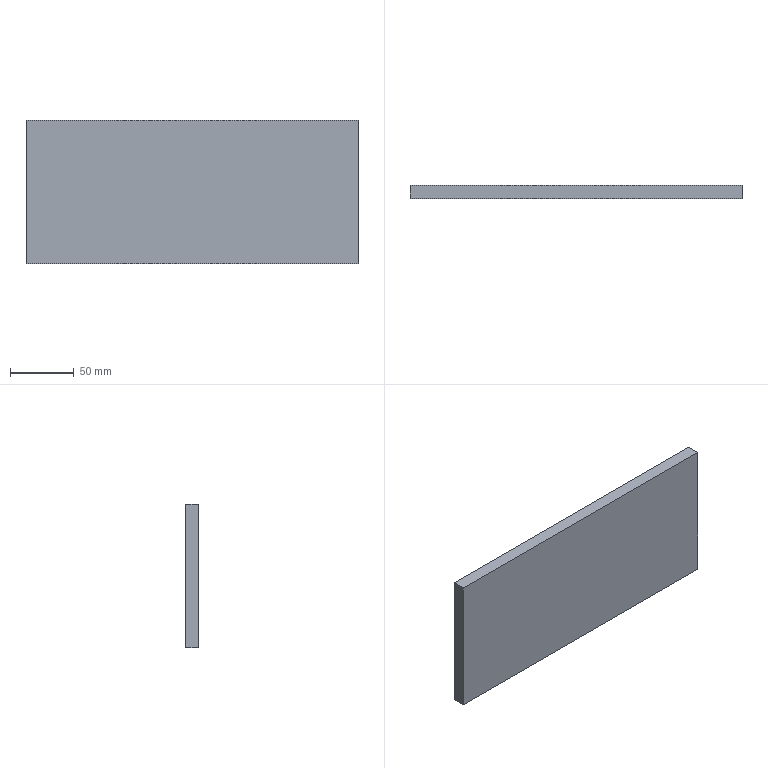Part | STEP file | Drawer | 1 solid | 6 faces | box 260 x 10 x 112 mm | volume 291200 mm3 | plane 6
STEP:
#1=CARTESIAN_POINT('',(0.,0.,0.));
#2=DIRECTION('',(0.,0.,1.));
#3=DIRECTION('',(1.,0.,0.));
#4=AXIS2_PLACEMENT_3D('',#1,#2,#3);
#5=CARTESIAN_POINT('',(-130.,0.,112.));
#6=VERTEX_POINT('',#5);
#7=CARTESIAN_POINT('',(-130.,-10.,112.));
#8=VERTEX_POINT('',#7);
#9=CARTESIAN_POINT('',(-130.,0.,112.));
#10=DIRECTION('',(0.,-1.,0.));
#11=VECTOR('',#10,1.);
#12=LINE('',#9,#11);
#13=CARTESIAN_POINT('',(-130.,0.,112.));
#14=DIRECTION('',(1.,0.,0.));
#15=DIRECTION('',(0.,0.,-1.));
#16=AXIS2_PLACEMENT_3D('',#13,#14,#15);
#17=PLANE('',#16);
#18=CARTESIAN_POINT('',(0.,0.));
#19=DIRECTION('',(0.,-1.));
#20=VECTOR('',#19,1.);
#21=LINE('',#18,#20);
#22=(GEOMETRIC_REPRESENTATION_CONTEXT(2)PARAMETRIC_REPRESENTATION_CONTEXT()REPRESENTATION_CONTEXT('',''));
#23=DEFINITIONAL_REPRESENTATION('',(#21),#22);
#24=PCURVE('',#17,#23);
#25=CARTESIAN_POINT('',(130.,0.,112.));
#26=DIRECTION('',(0.,0.,-1.));
#27=DIRECTION('',(-1.,0.,0.));
#28=AXIS2_PLACEMENT_3D('',#25,#26,#27);
#29=PLANE('',#28);
#30=CARTESIAN_POINT('',(260.,0.));
#31=DIRECTION('',(0.,-1.));
#32=VECTOR('',#31,1.);
#33=LINE('',#30,#32);
#34=(GEOMETRIC_REPRESENTATION_CONTEXT(2)PARAMETRIC_REPRESENTATION_CONTEXT()REPRESENTATION_CONTEXT('',''));
#35=DEFINITIONAL_REPRESENTATION('',(#33),#34);
#36=PCURVE('',#29,#35);
#37=SURFACE_CURVE('',#12,(#24,#36),.PCURVE_S1.);
#38=EDGE_CURVE('',#6,#8,#37,.T.);
#39=ORIENTED_EDGE('',*,*,#38,.T.);
#40=CARTESIAN_POINT('',(-130.,-10.,0.));
#41=VERTEX_POINT('',#40);
#42=CARTESIAN_POINT('',(-130.,-10.,112.));
#43=DIRECTION('',(0.,0.,-1.));
#44=VECTOR('',#43,1.);
#45=LINE('',#42,#44);
#46=CARTESIAN_POINT('',(0.,-10.));
#47=DIRECTION('',(1.,0.));
#48=VECTOR('',#47,1.);
#49=LINE('',#46,#48);
#50=(GEOMETRIC_REPRESENTATION_CONTEXT(2)PARAMETRIC_REPRESENTATION_CONTEXT()REPRESENTATION_CONTEXT('',''));
#51=DEFINITIONAL_REPRESENTATION('',(#49),#50);
#52=PCURVE('',#17,#51);
#53=CARTESIAN_POINT('',(0.,-10.,56.));
#54=DIRECTION('',(0.,1.,0.));
#55=DIRECTION('',(0.,0.,1.));
#56=AXIS2_PLACEMENT_3D('',#53,#54,#55);
#57=PLANE('',#56);
#58=CARTESIAN_POINT('',(56.,-130.));
#59=DIRECTION('',(-1.,0.));
#60=VECTOR('',#59,1.);
#61=LINE('',#58,#60);
#62=(GEOMETRIC_REPRESENTATION_CONTEXT(2)PARAMETRIC_REPRESENTATION_CONTEXT()REPRESENTATION_CONTEXT('',''));
#63=DEFINITIONAL_REPRESENTATION('',(#61),#62);
#64=PCURVE('',#57,#63);
#65=SURFACE_CURVE('',#45,(#52,#64),.PCURVE_S1.);
#66=EDGE_CURVE('',#8,#41,#65,.T.);
#67=ORIENTED_EDGE('',*,*,#66,.T.);
#68=CARTESIAN_POINT('',(-130.,0.,0.));
#69=VERTEX_POINT('',#68);
#70=CARTESIAN_POINT('',(-130.,0.,0.));
#71=DIRECTION('',(0.,-1.,0.));
#72=VECTOR('',#71,1.);
#73=LINE('',#70,#72);
#74=CARTESIAN_POINT('',(112.,0.));
#75=DIRECTION('',(0.,-1.));
#76=VECTOR('',#75,1.);
#77=LINE('',#74,#76);
#78=(GEOMETRIC_REPRESENTATION_CONTEXT(2)PARAMETRIC_REPRESENTATION_CONTEXT()REPRESENTATION_CONTEXT('',''));
#79=DEFINITIONAL_REPRESENTATION('',(#77),#78);
#80=PCURVE('',#17,#79);
#81=CARTESIAN_POINT('',(-130.,0.,0.));
#82=DIRECTION('',(0.,0.,1.));
#83=DIRECTION('',(1.,0.,0.));
#84=AXIS2_PLACEMENT_3D('',#81,#82,#83);
#85=PLANE('',#84);
#86=CARTESIAN_POINT('',(0.,0.));
#87=DIRECTION('',(0.,-1.));
#88=VECTOR('',#87,1.);
#89=LINE('',#86,#88);
#90=(GEOMETRIC_REPRESENTATION_CONTEXT(2)PARAMETRIC_REPRESENTATION_CONTEXT()REPRESENTATION_CONTEXT('',''));
#91=DEFINITIONAL_REPRESENTATION('',(#89),#90);
#92=PCURVE('',#85,#91);
#93=SURFACE_CURVE('',#73,(#80,#92),.PCURVE_S1.);
#94=EDGE_CURVE('',#69,#41,#93,.T.);
#95=ORIENTED_EDGE('',*,*,#94,.F.);
#96=CARTESIAN_POINT('',(-130.,0.,112.));
#97=DIRECTION('',(0.,0.,-1.));
#98=VECTOR('',#97,1.);
#99=LINE('',#96,#98);
#100=CARTESIAN_POINT('',(0.,0.));
#101=DIRECTION('',(1.,0.));
#102=VECTOR('',#101,1.);
#103=LINE('',#100,#102);
#104=(GEOMETRIC_REPRESENTATION_CONTEXT(2)PARAMETRIC_REPRESENTATION_CONTEXT()REPRESENTATION_CONTEXT('',''));
#105=DEFINITIONAL_REPRESENTATION('',(#103),#104);
#106=PCURVE('',#17,#105);
#107=CARTESIAN_POINT('',(0.,0.,56.));
#108=DIRECTION('',(0.,1.,0.));
#109=DIRECTION('',(0.,0.,1.));
#110=AXIS2_PLACEMENT_3D('',#107,#108,#109);
#111=PLANE('',#110);
#112=CARTESIAN_POINT('',(56.,-130.));
#113=DIRECTION('',(-1.,0.));
#114=VECTOR('',#113,1.);
#115=LINE('',#112,#114);
#116=(GEOMETRIC_REPRESENTATION_CONTEXT(2)PARAMETRIC_REPRESENTATION_CONTEXT()REPRESENTATION_CONTEXT('',''));
#117=DEFINITIONAL_REPRESENTATION('',(#115),#116);
#118=PCURVE('',#111,#117);
#119=SURFACE_CURVE('',#99,(#106,#118),.PCURVE_S1.);
#120=EDGE_CURVE('',#6,#69,#119,.T.);
#121=ORIENTED_EDGE('',*,*,#120,.F.);
#122=EDGE_LOOP('',(#39,#67,#95,#121));
#123=FACE_BOUND('',#122,.F.);
#124=ADVANCED_FACE('',(#123),#17,.F.);
#125=ORIENTED_EDGE('',*,*,#94,.T.);
#126=CARTESIAN_POINT('',(130.,-10.,0.));
#127=VERTEX_POINT('',#126);
#128=CARTESIAN_POINT('',(-130.,-10.,0.));
#129=DIRECTION('',(1.,0.,0.));
#130=VECTOR('',#129,1.);
#131=LINE('',#128,#130);
#132=CARTESIAN_POINT('',(0.,-10.));
#133=DIRECTION('',(1.,0.));
#134=VECTOR('',#133,1.);
#135=LINE('',#132,#134);
#136=(GEOMETRIC_REPRESENTATION_CONTEXT(2)PARAMETRIC_REPRESENTATION_CONTEXT()REPRESENTATION_CONTEXT('',''));
#137=DEFINITIONAL_REPRESENTATION('',(#135),#136);
#138=PCURVE('',#85,#137);
#139=CARTESIAN_POINT('',(-56.,-130.));
#140=DIRECTION('',(0.,1.));
#141=VECTOR('',#140,1.);
#142=LINE('',#139,#141);
#143=(GEOMETRIC_REPRESENTATION_CONTEXT(2)PARAMETRIC_REPRESENTATION_CONTEXT()REPRESENTATION_CONTEXT('',''));
#144=DEFINITIONAL_REPRESENTATION('',(#142),#143);
#145=PCURVE('',#57,#144);
#146=SURFACE_CURVE('',#131,(#138,#145),.PCURVE_S1.);
#147=EDGE_CURVE('',#41,#127,#146,.T.);
#148=ORIENTED_EDGE('',*,*,#147,.T.);
#149=CARTESIAN_POINT('',(130.,0.,0.));
#150=VERTEX_POINT('',#149);
#151=CARTESIAN_POINT('',(130.,0.,0.));
#152=DIRECTION('',(0.,-1.,0.));
#153=VECTOR('',#152,1.);
#154=LINE('',#151,#153);
#155=CARTESIAN_POINT('',(260.,0.));
#156=DIRECTION('',(0.,-1.));
#157=VECTOR('',#156,1.);
#158=LINE('',#155,#157);
#159=(GEOMETRIC_REPRESENTATION_CONTEXT(2)PARAMETRIC_REPRESENTATION_CONTEXT()REPRESENTATION_CONTEXT('',''));
#160=DEFINITIONAL_REPRESENTATION('',(#158),#159);
#161=PCURVE('',#85,#160);
#162=CARTESIAN_POINT('',(130.,0.,0.));
#163=DIRECTION('',(-1.,0.,0.));
#164=DIRECTION('',(0.,0.,1.));
#165=AXIS2_PLACEMENT_3D('',#162,#163,#164);
#166=PLANE('',#165);
#167=CARTESIAN_POINT('',(0.,0.));
#168=DIRECTION('',(0.,-1.));
#169=VECTOR('',#168,1.);
#170=LINE('',#167,#169);
#171=(GEOMETRIC_REPRESENTATION_CONTEXT(2)PARAMETRIC_REPRESENTATION_CONTEXT()REPRESENTATION_CONTEXT('',''));
#172=DEFINITIONAL_REPRESENTATION('',(#170),#171);
#173=PCURVE('',#166,#172);
#174=SURFACE_CURVE('',#154,(#161,#173),.PCURVE_S1.);
#175=EDGE_CURVE('',#150,#127,#174,.T.);
#176=ORIENTED_EDGE('',*,*,#175,.F.);
#177=CARTESIAN_POINT('',(-130.,0.,0.));
#178=DIRECTION('',(1.,0.,0.));
#179=VECTOR('',#178,1.);
#180=LINE('',#177,#179);
#181=CARTESIAN_POINT('',(0.,0.));
#182=DIRECTION('',(1.,0.));
#183=VECTOR('',#182,1.);
#184=LINE('',#181,#183);
#185=(GEOMETRIC_REPRESENTATION_CONTEXT(2)PARAMETRIC_REPRESENTATION_CONTEXT()REPRESENTATION_CONTEXT('',''));
#186=DEFINITIONAL_REPRESENTATION('',(#184),#185);
#187=PCURVE('',#85,#186);
#188=CARTESIAN_POINT('',(-56.,-130.));
#189=DIRECTION('',(0.,1.));
#190=VECTOR('',#189,1.);
#191=LINE('',#188,#190);
#192=(GEOMETRIC_REPRESENTATION_CONTEXT(2)PARAMETRIC_REPRESENTATION_CONTEXT()REPRESENTATION_CONTEXT('',''));
#193=DEFINITIONAL_REPRESENTATION('',(#191),#192);
#194=PCURVE('',#111,#193);
#195=SURFACE_CURVE('',#180,(#187,#194),.PCURVE_S1.);
#196=EDGE_CURVE('',#69,#150,#195,.T.);
#197=ORIENTED_EDGE('',*,*,#196,.F.);
#198=EDGE_LOOP('',(#125,#148,#176,#197));
#199=FACE_BOUND('',#198,.F.);
#200=ADVANCED_FACE('',(#199),#85,.F.);
#201=ORIENTED_EDGE('',*,*,#175,.T.);
#202=CARTESIAN_POINT('',(130.,-10.,112.));
#203=VERTEX_POINT('',#202);
#204=CARTESIAN_POINT('',(130.,-10.,0.));
#205=DIRECTION('',(0.,0.,1.));
#206=VECTOR('',#205,1.);
#207=LINE('',#204,#206);
#208=CARTESIAN_POINT('',(0.,-10.));
#209=DIRECTION('',(1.,0.));
#210=VECTOR('',#209,1.);
#211=LINE('',#208,#210);
#212=(GEOMETRIC_REPRESENTATION_CONTEXT(2)PARAMETRIC_REPRESENTATION_CONTEXT()REPRESENTATION_CONTEXT('',''));
#213=DEFINITIONAL_REPRESENTATION('',(#211),#212);
#214=PCURVE('',#166,#213);
#215=CARTESIAN_POINT('',(-56.,130.));
#216=DIRECTION('',(1.,0.));
#217=VECTOR('',#216,1.);
#218=LINE('',#215,#217);
#219=(GEOMETRIC_REPRESENTATION_CONTEXT(2)PARAMETRIC_REPRESENTATION_CONTEXT()REPRESENTATION_CONTEXT('',''));
#220=DEFINITIONAL_REPRESENTATION('',(#218),#219);
#221=PCURVE('',#57,#220);
#222=SURFACE_CURVE('',#207,(#214,#221),.PCURVE_S1.);
#223=EDGE_CURVE('',#127,#203,#222,.T.);
#224=ORIENTED_EDGE('',*,*,#223,.T.);
#225=CARTESIAN_POINT('',(130.,0.,112.));
#226=VERTEX_POINT('',#225);
#227=CARTESIAN_POINT('',(130.,0.,112.));
#228=DIRECTION('',(0.,-1.,0.));
#229=VECTOR('',#228,1.);
#230=LINE('',#227,#229);
#231=CARTESIAN_POINT('',(112.,0.));
#232=DIRECTION('',(0.,-1.));
#233=VECTOR('',#232,1.);
#234=LINE('',#231,#233);
#235=(GEOMETRIC_REPRESENTATION_CONTEXT(2)PARAMETRIC_REPRESENTATION_CONTEXT()REPRESENTATION_CONTEXT('',''));
#236=DEFINITIONAL_REPRESENTATION('',(#234),#235);
#237=PCURVE('',#166,#236);
#238=CARTESIAN_POINT('',(0.,0.));
#239=DIRECTION('',(0.,-1.));
#240=VECTOR('',#239,1.);
#241=LINE('',#238,#240);
#242=(GEOMETRIC_REPRESENTATION_CONTEXT(2)PARAMETRIC_REPRESENTATION_CONTEXT()REPRESENTATION_CONTEXT('',''));
#243=DEFINITIONAL_REPRESENTATION('',(#241),#242);
#244=PCURVE('',#29,#243);
#245=SURFACE_CURVE('',#230,(#237,#244),.PCURVE_S1.);
#246=EDGE_CURVE('',#226,#203,#245,.T.);
#247=ORIENTED_EDGE('',*,*,#246,.F.);
#248=CARTESIAN_POINT('',(130.,0.,0.));
#249=DIRECTION('',(0.,0.,1.));
#250=VECTOR('',#249,1.);
#251=LINE('',#248,#250);
#252=CARTESIAN_POINT('',(0.,0.));
#253=DIRECTION('',(1.,0.));
#254=VECTOR('',#253,1.);
#255=LINE('',#252,#254);
#256=(GEOMETRIC_REPRESENTATION_CONTEXT(2)PARAMETRIC_REPRESENTATION_CONTEXT()REPRESENTATION_CONTEXT('',''));
#257=DEFINITIONAL_REPRESENTATION('',(#255),#256);
#258=PCURVE('',#166,#257);
#259=CARTESIAN_POINT('',(-56.,130.));
#260=DIRECTION('',(1.,0.));
#261=VECTOR('',#260,1.);
#262=LINE('',#259,#261);
#263=(GEOMETRIC_REPRESENTATION_CONTEXT(2)PARAMETRIC_REPRESENTATION_CONTEXT()REPRESENTATION_CONTEXT('',''));
#264=DEFINITIONAL_REPRESENTATION('',(#262),#263);
#265=PCURVE('',#111,#264);
#266=SURFACE_CURVE('',#251,(#258,#265),.PCURVE_S1.);
#267=EDGE_CURVE('',#150,#226,#266,.T.);
#268=ORIENTED_EDGE('',*,*,#267,.F.);
#269=EDGE_LOOP('',(#201,#224,#247,#268));
#270=FACE_BOUND('',#269,.F.);
#271=ADVANCED_FACE('',(#270),#166,.F.);
#272=ORIENTED_EDGE('',*,*,#246,.T.);
#273=CARTESIAN_POINT('',(130.,-10.,112.));
#274=DIRECTION('',(-1.,0.,0.));
#275=VECTOR('',#274,1.);
#276=LINE('',#273,#275);
#277=CARTESIAN_POINT('',(0.,-10.));
#278=DIRECTION('',(1.,0.));
#279=VECTOR('',#278,1.);
#280=LINE('',#277,#279);
#281=(GEOMETRIC_REPRESENTATION_CONTEXT(2)PARAMETRIC_REPRESENTATION_CONTEXT()REPRESENTATION_CONTEXT('',''));
#282=DEFINITIONAL_REPRESENTATION('',(#280),#281);
#283=PCURVE('',#29,#282);
#284=CARTESIAN_POINT('',(56.,130.));
#285=DIRECTION('',(0.,-1.));
#286=VECTOR('',#285,1.);
#287=LINE('',#284,#286);
#288=(GEOMETRIC_REPRESENTATION_CONTEXT(2)PARAMETRIC_REPRESENTATION_CONTEXT()REPRESENTATION_CONTEXT('',''));
#289=DEFINITIONAL_REPRESENTATION('',(#287),#288);
#290=PCURVE('',#57,#289);
#291=SURFACE_CURVE('',#276,(#283,#290),.PCURVE_S1.);
#292=EDGE_CURVE('',#203,#8,#291,.T.);
#293=ORIENTED_EDGE('',*,*,#292,.T.);
#294=ORIENTED_EDGE('',*,*,#38,.F.);
#295=CARTESIAN_POINT('',(130.,0.,112.));
#296=DIRECTION('',(-1.,0.,0.));
#297=VECTOR('',#296,1.);
#298=LINE('',#295,#297);
#299=CARTESIAN_POINT('',(0.,0.));
#300=DIRECTION('',(1.,0.));
#301=VECTOR('',#300,1.);
#302=LINE('',#299,#301);
#303=(GEOMETRIC_REPRESENTATION_CONTEXT(2)PARAMETRIC_REPRESENTATION_CONTEXT()REPRESENTATION_CONTEXT('',''));
#304=DEFINITIONAL_REPRESENTATION('',(#302),#303);
#305=PCURVE('',#29,#304);
#306=CARTESIAN_POINT('',(56.,130.));
#307=DIRECTION('',(0.,-1.));
#308=VECTOR('',#307,1.);
#309=LINE('',#306,#308);
#310=(GEOMETRIC_REPRESENTATION_CONTEXT(2)PARAMETRIC_REPRESENTATION_CONTEXT()REPRESENTATION_CONTEXT('',''));
#311=DEFINITIONAL_REPRESENTATION('',(#309),#310);
#312=PCURVE('',#111,#311);
#313=SURFACE_CURVE('',#298,(#305,#312),.PCURVE_S1.);
#314=EDGE_CURVE('',#226,#6,#313,.T.);
#315=ORIENTED_EDGE('',*,*,#314,.F.);
#316=EDGE_LOOP('',(#272,#293,#294,#315));
#317=FACE_BOUND('',#316,.F.);
#318=ADVANCED_FACE('',(#317),#29,.F.);
#319=ORIENTED_EDGE('',*,*,#120,.T.);
#320=ORIENTED_EDGE('',*,*,#196,.T.);
#321=ORIENTED_EDGE('',*,*,#267,.T.);
#322=ORIENTED_EDGE('',*,*,#314,.T.);
#323=EDGE_LOOP('',(#319,#320,#321,#322));
#324=FACE_BOUND('',#323,.F.);
#325=ADVANCED_FACE('',(#324),#111,.T.);
#326=ORIENTED_EDGE('',*,*,#66,.T.);
#327=ORIENTED_EDGE('',*,*,#147,.T.);
#328=ORIENTED_EDGE('',*,*,#223,.T.);
#329=ORIENTED_EDGE('',*,*,#292,.T.);
#330=EDGE_LOOP('',(#326,#327,#328,#329));
#331=FACE_BOUND('',#330,.T.);
#332=ADVANCED_FACE('',(#331),#57,.F.);
#333=CLOSED_SHELL('',(#124,#200,#271,#318,#325,#332));
#334=MANIFOLD_SOLID_BREP('',#333);
#335=(LENGTH_UNIT()NAMED_UNIT(*)SI_UNIT(.MILLI.,.METRE.));
#336=UNCERTAINTY_MEASURE_WITH_UNIT(LENGTH_MEASURE(0.0000001),#335,'','');
#337=(NAMED_UNIT(*)PLANE_ANGLE_UNIT()SI_UNIT($,.RADIAN.));
#338=(NAMED_UNIT(*)SI_UNIT($,.STERADIAN.)SOLID_ANGLE_UNIT());
#339=(GEOMETRIC_REPRESENTATION_CONTEXT(3)GLOBAL_UNCERTAINTY_ASSIGNED_CONTEXT((#336))GLOBAL_UNIT_ASSIGNED_CONTEXT((#335,#337,#338))REPRESENTATION_CONTEXT('',''));
#340=ADVANCED_BREP_SHAPE_REPRESENTATION('',(#4,#334),#339);